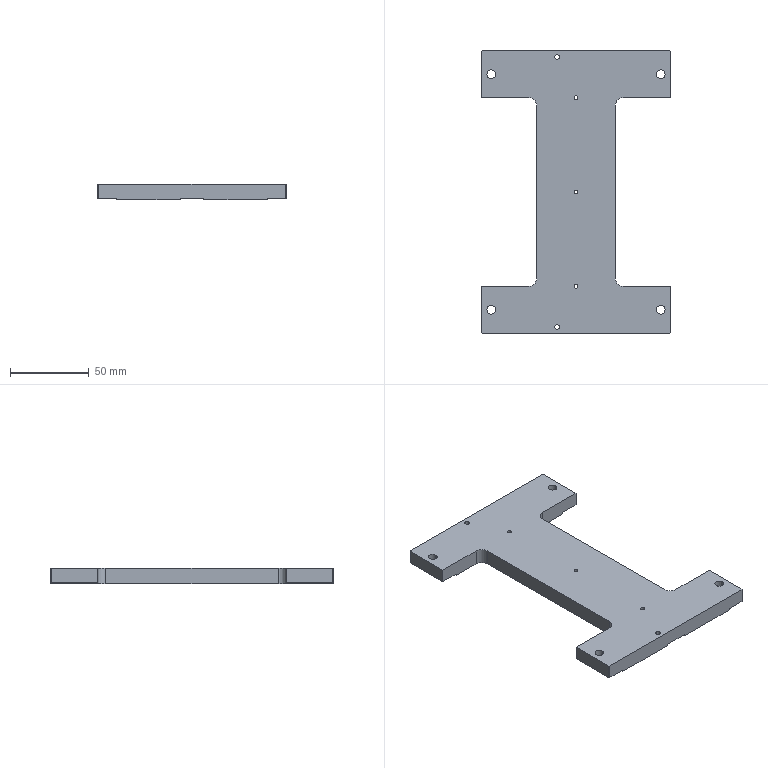Part | STEP file | 2067 Gripper mounting plate | 1 solid | 52 faces | box 120 x 180 x 10 mm | volume 126941 mm3 | plane 30 | cylinder 22 | commonest cylinder face diameters 5.5 x8 2.5 x6 3 x4 10 x4